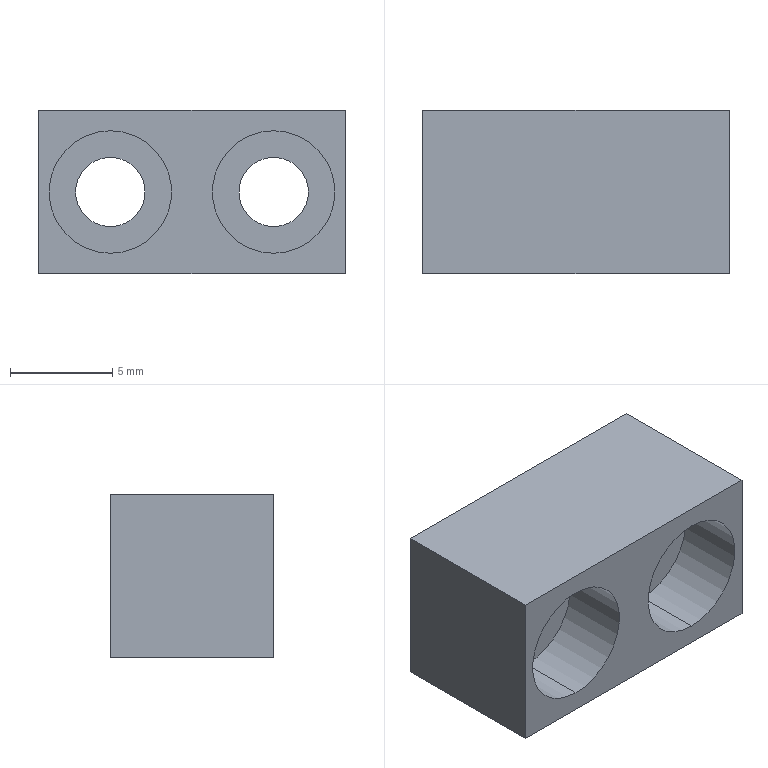Part | NX | features BREP 1 | 1 solid | 19 faces | box 15 x 8 x 8 mm | volume 660.349 mm3 | cylinder 10 | plane 9 | commonest cylinder face diameters 3.4 x4 6 x4 4.5 x2
STEP:
#1=CARTESIAN_POINT('',(4.,-0.6,3.));
#2=VERTEX_POINT('',#1);
#3=CARTESIAN_POINT('',(4.,-0.6,-3.));
#4=VERTEX_POINT('',#3);
#5=CARTESIAN_POINT('',(4.,-0.6,0.));
#6=DIRECTION('',(0.,-1.,0.));
#7=DIRECTION('',(0.,0.,-1.));
#8=AXIS2_PLACEMENT_3D('',#5,#6,#7);
#9=CIRCLE('',#8,3.);
#10=EDGE_CURVE('',#2,#4,#9,.T.);
#11=ORIENTED_EDGE('',*,*,#10,.F.);
#12=CARTESIAN_POINT('',(4.,-4.,3.));
#13=VERTEX_POINT('',#12);
#14=CARTESIAN_POINT('',(4.,-4.,3.));
#15=DIRECTION('',(0.,-1.,0.));
#16=VECTOR('',#15,1000.);
#17=LINE('',#14,#16);
#18=EDGE_CURVE('',#13,#2,#17,.F.);
#19=ORIENTED_EDGE('',*,*,#18,.F.);
#20=CARTESIAN_POINT('',(4.,-4.,-3.));
#21=VERTEX_POINT('',#20);
#22=CARTESIAN_POINT('',(4.,-4.,0.));
#23=DIRECTION('',(0.,-1.,0.));
#24=DIRECTION('',(0.,0.,-1.));
#25=AXIS2_PLACEMENT_3D('',#22,#23,#24);
#26=CIRCLE('',#25,3.);
#27=EDGE_CURVE('',#13,#21,#26,.T.);
#28=ORIENTED_EDGE('',*,*,#27,.T.);
#29=CARTESIAN_POINT('',(4.,-4.,-3.));
#30=DIRECTION('',(0.,-1.,0.));
#31=VECTOR('',#30,1000.);
#32=LINE('',#29,#31);
#33=EDGE_CURVE('',#21,#4,#32,.F.);
#34=ORIENTED_EDGE('',*,*,#33,.T.);
#35=EDGE_LOOP('',(#11,#19,#28,#34));
#36=FACE_BOUND('',#35,.T.);
#37=CARTESIAN_POINT('',(4.,-4.,0.));
#38=DIRECTION('',(0.,-1.,0.));
#39=DIRECTION('',(0.,0.,1.));
#40=AXIS2_PLACEMENT_3D('',#37,#38,#39);
#41=CYLINDRICAL_SURFACE('',#40,3.);
#42=ADVANCED_FACE('',(#36),#41,.F.);
#43=CARTESIAN_POINT('',(4.,4.,1.7));
#44=VERTEX_POINT('',#43);
#45=CARTESIAN_POINT('',(4.,4.,-1.7));
#46=VERTEX_POINT('',#45);
#47=CARTESIAN_POINT('',(4.,4.,0.));
#48=DIRECTION('',(0.,-1.,0.));
#49=DIRECTION('',(0.,0.,-1.));
#50=AXIS2_PLACEMENT_3D('',#47,#48,#49);
#51=CIRCLE('',#50,1.7);
#52=EDGE_CURVE('',#44,#46,#51,.T.);
#53=ORIENTED_EDGE('',*,*,#52,.F.);
#54=CARTESIAN_POINT('',(4.,-0.6,1.7));
#55=VERTEX_POINT('',#54);
#56=CARTESIAN_POINT('',(4.,-4.,1.7));
#57=DIRECTION('',(0.,-1.,0.));
#58=VECTOR('',#57,1000.);
#59=LINE('',#56,#58);
#60=EDGE_CURVE('',#55,#44,#59,.F.);
#61=ORIENTED_EDGE('',*,*,#60,.F.);
#62=CARTESIAN_POINT('',(4.,-0.6,-1.7));
#63=VERTEX_POINT('',#62);
#64=CARTESIAN_POINT('',(4.,-0.6,0.));
#65=DIRECTION('',(0.,-1.,0.));
#66=DIRECTION('',(0.,0.,-1.));
#67=AXIS2_PLACEMENT_3D('',#64,#65,#66);
#68=CIRCLE('',#67,1.7);
#69=EDGE_CURVE('',#55,#63,#68,.T.);
#70=ORIENTED_EDGE('',*,*,#69,.T.);
#71=CARTESIAN_POINT('',(4.,-4.,-1.7));
#72=DIRECTION('',(0.,-1.,0.));
#73=VECTOR('',#72,1000.);
#74=LINE('',#71,#73);
#75=EDGE_CURVE('',#63,#46,#74,.F.);
#76=ORIENTED_EDGE('',*,*,#75,.T.);
#77=EDGE_LOOP('',(#53,#61,#70,#76));
#78=FACE_BOUND('',#77,.T.);
#79=CARTESIAN_POINT('',(4.,-4.,0.));
#80=DIRECTION('',(0.,-1.,0.));
#81=DIRECTION('',(0.,0.,1.));
#82=AXIS2_PLACEMENT_3D('',#79,#80,#81);
#83=CYLINDRICAL_SURFACE('',#82,1.7);
#84=ADVANCED_FACE('',(#78),#83,.F.);
#85=CARTESIAN_POINT('',(-4.,-0.6,3.));
#86=VERTEX_POINT('',#85);
#87=CARTESIAN_POINT('',(-4.,-0.6,-3.));
#88=VERTEX_POINT('',#87);
#89=CARTESIAN_POINT('',(-4.,-0.6,0.));
#90=DIRECTION('',(0.,-1.,0.));
#91=DIRECTION('',(0.,0.,-1.));
#92=AXIS2_PLACEMENT_3D('',#89,#90,#91);
#93=CIRCLE('',#92,3.);
#94=EDGE_CURVE('',#86,#88,#93,.T.);
#95=ORIENTED_EDGE('',*,*,#94,.F.);
#96=CARTESIAN_POINT('',(-4.,-4.,3.));
#97=VERTEX_POINT('',#96);
#98=CARTESIAN_POINT('',(-4.,-4.,3.));
#99=DIRECTION('',(0.,-1.,0.));
#100=VECTOR('',#99,1000.);
#101=LINE('',#98,#100);
#102=EDGE_CURVE('',#97,#86,#101,.F.);
#103=ORIENTED_EDGE('',*,*,#102,.F.);
#104=CARTESIAN_POINT('',(-4.,-4.,-3.));
#105=VERTEX_POINT('',#104);
#106=CARTESIAN_POINT('',(-4.,-4.,0.));
#107=DIRECTION('',(0.,-1.,0.));
#108=DIRECTION('',(0.,0.,-1.));
#109=AXIS2_PLACEMENT_3D('',#106,#107,#108);
#110=CIRCLE('',#109,3.);
#111=EDGE_CURVE('',#97,#105,#110,.T.);
#112=ORIENTED_EDGE('',*,*,#111,.T.);
#113=CARTESIAN_POINT('',(-4.,-4.,-3.));
#114=DIRECTION('',(0.,-1.,0.));
#115=VECTOR('',#114,1000.);
#116=LINE('',#113,#115);
#117=EDGE_CURVE('',#105,#88,#116,.F.);
#118=ORIENTED_EDGE('',*,*,#117,.T.);
#119=EDGE_LOOP('',(#95,#103,#112,#118));
#120=FACE_BOUND('',#119,.T.);
#121=CARTESIAN_POINT('',(-4.,-4.,0.));
#122=DIRECTION('',(0.,-1.,0.));
#123=DIRECTION('',(0.,0.,1.));
#124=AXIS2_PLACEMENT_3D('',#121,#122,#123);
#125=CYLINDRICAL_SURFACE('',#124,3.);
#126=ADVANCED_FACE('',(#120),#125,.F.);
#127=CARTESIAN_POINT('',(-4.,4.,1.7));
#128=VERTEX_POINT('',#127);
#129=CARTESIAN_POINT('',(-4.,4.,-1.7));
#130=VERTEX_POINT('',#129);
#131=CARTESIAN_POINT('',(-4.,4.,0.));
#132=DIRECTION('',(0.,-1.,0.));
#133=DIRECTION('',(0.,0.,-1.));
#134=AXIS2_PLACEMENT_3D('',#131,#132,#133);
#135=CIRCLE('',#134,1.7);
#136=EDGE_CURVE('',#128,#130,#135,.T.);
#137=ORIENTED_EDGE('',*,*,#136,.F.);
#138=CARTESIAN_POINT('',(-4.,-0.6,1.7));
#139=VERTEX_POINT('',#138);
#140=CARTESIAN_POINT('',(-4.,-4.,1.7));
#141=DIRECTION('',(0.,-1.,0.));
#142=VECTOR('',#141,1000.);
#143=LINE('',#140,#142);
#144=EDGE_CURVE('',#139,#128,#143,.F.);
#145=ORIENTED_EDGE('',*,*,#144,.F.);
#146=CARTESIAN_POINT('',(-4.,-0.6,-1.7));
#147=VERTEX_POINT('',#146);
#148=CARTESIAN_POINT('',(-4.,-0.6,0.));
#149=DIRECTION('',(0.,-1.,0.));
#150=DIRECTION('',(0.,0.,-1.));
#151=AXIS2_PLACEMENT_3D('',#148,#149,#150);
#152=CIRCLE('',#151,1.7);
#153=EDGE_CURVE('',#139,#147,#152,.T.);
#154=ORIENTED_EDGE('',*,*,#153,.T.);
#155=CARTESIAN_POINT('',(-4.,-4.,-1.7));
#156=DIRECTION('',(0.,-1.,0.));
#157=VECTOR('',#156,1000.);
#158=LINE('',#155,#157);
#159=EDGE_CURVE('',#147,#130,#158,.F.);
#160=ORIENTED_EDGE('',*,*,#159,.T.);
#161=EDGE_LOOP('',(#137,#145,#154,#160));
#162=FACE_BOUND('',#161,.T.);
#163=CARTESIAN_POINT('',(-4.,-4.,0.));
#164=DIRECTION('',(0.,-1.,0.));
#165=DIRECTION('',(0.,0.,1.));
#166=AXIS2_PLACEMENT_3D('',#163,#164,#165);
#167=CYLINDRICAL_SURFACE('',#166,1.7);
#168=ADVANCED_FACE('',(#162),#167,.F.);
#169=CARTESIAN_POINT('',(2.25,1.,-2.5));
#170=VERTEX_POINT('',#169);
#171=CARTESIAN_POINT('',(-2.25,1.,-2.5));
#172=VERTEX_POINT('',#171);
#173=CARTESIAN_POINT('',(0.,1.,-2.5));
#174=DIRECTION('',(0.,0.,-1.));
#175=DIRECTION('',(-1.,0.,0.));
#176=AXIS2_PLACEMENT_3D('',#173,#174,#175);
#177=CIRCLE('',#176,2.25);
#178=EDGE_CURVE('',#170,#172,#177,.T.);
#179=ORIENTED_EDGE('',*,*,#178,.F.);
#180=CARTESIAN_POINT('',(2.25,1.,-4.));
#181=VERTEX_POINT('',#180);
#182=CARTESIAN_POINT('',(2.25,1.,-2.5));
#183=DIRECTION('',(0.,0.,-1.));
#184=VECTOR('',#183,1000.);
#185=LINE('',#182,#184);
#186=EDGE_CURVE('',#181,#170,#185,.F.);
#187=ORIENTED_EDGE('',*,*,#186,.F.);
#188=CARTESIAN_POINT('',(-2.25,1.,-4.));
#189=VERTEX_POINT('',#188);
#190=CARTESIAN_POINT('',(0.,1.,-4.));
#191=DIRECTION('',(0.,0.,-1.));
#192=DIRECTION('',(-1.,0.,0.));
#193=AXIS2_PLACEMENT_3D('',#190,#191,#192);
#194=CIRCLE('',#193,2.25);
#195=EDGE_CURVE('',#181,#189,#194,.T.);
#196=ORIENTED_EDGE('',*,*,#195,.T.);
#197=CARTESIAN_POINT('',(-2.25,1.,-2.5));
#198=DIRECTION('',(0.,0.,-1.));
#199=VECTOR('',#198,1000.);
#200=LINE('',#197,#199);
#201=EDGE_CURVE('',#189,#172,#200,.F.);
#202=ORIENTED_EDGE('',*,*,#201,.T.);
#203=EDGE_LOOP('',(#179,#187,#196,#202));
#204=FACE_BOUND('',#203,.T.);
#205=CARTESIAN_POINT('',(0.,1.,-2.5));
#206=DIRECTION('',(0.,0.,-1.));
#207=DIRECTION('',(1.,0.,0.));
#208=AXIS2_PLACEMENT_3D('',#205,#206,#207);
#209=CYLINDRICAL_SURFACE('',#208,2.25);
#210=ADVANCED_FACE('',(#204),#209,.F.);
#211=CARTESIAN_POINT('',(7.5,-4.,-4.));
#212=VERTEX_POINT('',#211);
#213=CARTESIAN_POINT('',(7.5,4.,-4.));
#214=VERTEX_POINT('',#213);
#215=CARTESIAN_POINT('',(7.5,4.,-4.));
#216=DIRECTION('',(0.,1.,0.));
#217=VECTOR('',#216,1000.);
#218=LINE('',#215,#217);
#219=EDGE_CURVE('',#212,#214,#218,.T.);
#220=ORIENTED_EDGE('',*,*,#219,.T.);
#221=CARTESIAN_POINT('',(7.5,4.,4.));
#222=VERTEX_POINT('',#221);
#223=CARTESIAN_POINT('',(7.5,4.,4.));
#224=DIRECTION('',(0.,0.,-1.));
#225=VECTOR('',#224,1000.);
#226=LINE('',#223,#225);
#227=EDGE_CURVE('',#222,#214,#226,.T.);
#228=ORIENTED_EDGE('',*,*,#227,.F.);
#229=CARTESIAN_POINT('',(7.5,-4.,4.));
#230=VERTEX_POINT('',#229);
#231=CARTESIAN_POINT('',(7.5,4.,4.));
#232=DIRECTION('',(0.,1.,0.));
#233=VECTOR('',#232,1000.);
#234=LINE('',#231,#233);
#235=EDGE_CURVE('',#230,#222,#234,.T.);
#236=ORIENTED_EDGE('',*,*,#235,.F.);
#237=CARTESIAN_POINT('',(7.5,-4.,4.));
#238=DIRECTION('',(0.,0.,-1.));
#239=VECTOR('',#238,1000.);
#240=LINE('',#237,#239);
#241=EDGE_CURVE('',#230,#212,#240,.T.);
#242=ORIENTED_EDGE('',*,*,#241,.T.);
#243=EDGE_LOOP('',(#220,#228,#236,#242));
#244=FACE_BOUND('',#243,.T.);
#245=CARTESIAN_POINT('',(7.5,4.,4.));
#246=DIRECTION('',(-1.,0.,0.));
#247=DIRECTION('',(0.,0.,-1.));
#248=AXIS2_PLACEMENT_3D('',#245,#246,#247);
#249=PLANE('',#248);
#250=ADVANCED_FACE('',(#244),#249,.F.);
#251=CARTESIAN_POINT('',(4.,4.,0.));
#252=DIRECTION('',(0.,-1.,0.));
#253=DIRECTION('',(0.,0.,-1.));
#254=AXIS2_PLACEMENT_3D('',#251,#252,#253);
#255=CIRCLE('',#254,1.7);
#256=EDGE_CURVE('',#46,#44,#255,.T.);
#257=ORIENTED_EDGE('',*,*,#256,.T.);
#258=ORIENTED_EDGE('',*,*,#52,.T.);
#259=EDGE_LOOP('',(#257,#258));
#260=FACE_BOUND('',#259,.T.);
#261=CARTESIAN_POINT('',(-4.,4.,0.));
#262=DIRECTION('',(0.,-1.,0.));
#263=DIRECTION('',(0.,0.,-1.));
#264=AXIS2_PLACEMENT_3D('',#261,#262,#263);
#265=CIRCLE('',#264,1.7);
#266=EDGE_CURVE('',#130,#128,#265,.T.);
#267=ORIENTED_EDGE('',*,*,#266,.T.);
#268=ORIENTED_EDGE('',*,*,#136,.T.);
#269=EDGE_LOOP('',(#267,#268));
#270=FACE_BOUND('',#269,.T.);
#271=CARTESIAN_POINT('',(-7.5,4.,-4.));
#272=VERTEX_POINT('',#271);
#273=CARTESIAN_POINT('',(-7.5,4.,-4.));
#274=DIRECTION('',(-1.,0.,0.));
#275=VECTOR('',#274,1000.);
#276=LINE('',#273,#275);
#277=EDGE_CURVE('',#214,#272,#276,.T.);
#278=ORIENTED_EDGE('',*,*,#277,.T.);
#279=CARTESIAN_POINT('',(-7.5,4.,4.));
#280=VERTEX_POINT('',#279);
#281=CARTESIAN_POINT('',(-7.5,4.,4.));
#282=DIRECTION('',(0.,0.,-1.));
#283=VECTOR('',#282,1000.);
#284=LINE('',#281,#283);
#285=EDGE_CURVE('',#280,#272,#284,.T.);
#286=ORIENTED_EDGE('',*,*,#285,.F.);
#287=CARTESIAN_POINT('',(-7.5,4.,4.));
#288=DIRECTION('',(-1.,0.,0.));
#289=VECTOR('',#288,1000.);
#290=LINE('',#287,#289);
#291=EDGE_CURVE('',#222,#280,#290,.T.);
#292=ORIENTED_EDGE('',*,*,#291,.F.);
#293=ORIENTED_EDGE('',*,*,#227,.T.);
#294=EDGE_LOOP('',(#278,#286,#292,#293));
#295=FACE_BOUND('',#294,.T.);
#296=CARTESIAN_POINT('',(-7.5,4.,4.));
#297=DIRECTION('',(0.,-1.,0.));
#298=DIRECTION('',(0.,0.,1.));
#299=AXIS2_PLACEMENT_3D('',#296,#297,#298);
#300=PLANE('',#299);
#301=ADVANCED_FACE('',(#260,#270,#295),#300,.F.);
#302=CARTESIAN_POINT('',(-7.5,-4.,-4.));
#303=VERTEX_POINT('',#302);
#304=CARTESIAN_POINT('',(-7.5,4.,-4.));
#305=DIRECTION('',(0.,-1.,0.));
#306=VECTOR('',#305,1000.);
#307=LINE('',#304,#306);
#308=EDGE_CURVE('',#272,#303,#307,.T.);
#309=ORIENTED_EDGE('',*,*,#308,.T.);
#310=CARTESIAN_POINT('',(-7.5,-4.,4.));
#311=VERTEX_POINT('',#310);
#312=CARTESIAN_POINT('',(-7.5,-4.,4.));
#313=DIRECTION('',(0.,0.,-1.));
#314=VECTOR('',#313,1000.);
#315=LINE('',#312,#314);
#316=EDGE_CURVE('',#311,#303,#315,.T.);
#317=ORIENTED_EDGE('',*,*,#316,.F.);
#318=CARTESIAN_POINT('',(-7.5,4.,4.));
#319=DIRECTION('',(0.,-1.,0.));
#320=VECTOR('',#319,1000.);
#321=LINE('',#318,#320);
#322=EDGE_CURVE('',#280,#311,#321,.T.);
#323=ORIENTED_EDGE('',*,*,#322,.F.);
#324=ORIENTED_EDGE('',*,*,#285,.T.);
#325=EDGE_LOOP('',(#309,#317,#323,#324));
#326=FACE_BOUND('',#325,.T.);
#327=CARTESIAN_POINT('',(-7.5,4.,4.));
#328=DIRECTION('',(1.,0.,0.));
#329=DIRECTION('',(0.,-1.,0.));
#330=AXIS2_PLACEMENT_3D('',#327,#328,#329);
#331=PLANE('',#330);
#332=ADVANCED_FACE('',(#326),#331,.F.);
#333=CARTESIAN_POINT('',(4.,-4.,0.));
#334=DIRECTION('',(0.,-1.,0.));
#335=DIRECTION('',(0.,0.,-1.));
#336=AXIS2_PLACEMENT_3D('',#333,#334,#335);
#337=CIRCLE('',#336,3.);
#338=EDGE_CURVE('',#21,#13,#337,.T.);
#339=ORIENTED_EDGE('',*,*,#338,.F.);
#340=ORIENTED_EDGE('',*,*,#27,.F.);
#341=EDGE_LOOP('',(#339,#340));
#342=FACE_BOUND('',#341,.T.);
#343=CARTESIAN_POINT('',(-4.,-4.,0.));
#344=DIRECTION('',(0.,-1.,0.));
#345=DIRECTION('',(0.,0.,-1.));
#346=AXIS2_PLACEMENT_3D('',#343,#344,#345);
#347=CIRCLE('',#346,3.);
#348=EDGE_CURVE('',#105,#97,#347,.T.);
#349=ORIENTED_EDGE('',*,*,#348,.F.);
#350=ORIENTED_EDGE('',*,*,#111,.F.);
#351=EDGE_LOOP('',(#349,#350));
#352=FACE_BOUND('',#351,.T.);
#353=CARTESIAN_POINT('',(-7.5,-4.,-4.));
#354=DIRECTION('',(1.,0.,0.));
#355=VECTOR('',#354,1000.);
#356=LINE('',#353,#355);
#357=EDGE_CURVE('',#303,#212,#356,.T.);
#358=ORIENTED_EDGE('',*,*,#357,.T.);
#359=ORIENTED_EDGE('',*,*,#241,.F.);
#360=CARTESIAN_POINT('',(-7.5,-4.,4.));
#361=DIRECTION('',(1.,0.,0.));
#362=VECTOR('',#361,1000.);
#363=LINE('',#360,#362);
#364=EDGE_CURVE('',#311,#230,#363,.T.);
#365=ORIENTED_EDGE('',*,*,#364,.F.);
#366=ORIENTED_EDGE('',*,*,#316,.T.);
#367=EDGE_LOOP('',(#358,#359,#365,#366));
#368=FACE_BOUND('',#367,.T.);
#369=CARTESIAN_POINT('',(-7.5,-4.,4.));
#370=DIRECTION('',(0.,1.,0.));
#371=DIRECTION('',(0.,0.,-1.));
#372=AXIS2_PLACEMENT_3D('',#369,#370,#371);
#373=PLANE('',#372);
#374=ADVANCED_FACE('',(#342,#352,#368),#373,.F.);
#375=ORIENTED_EDGE('',*,*,#235,.T.);
#376=ORIENTED_EDGE('',*,*,#291,.T.);
#377=ORIENTED_EDGE('',*,*,#322,.T.);
#378=ORIENTED_EDGE('',*,*,#364,.T.);
#379=EDGE_LOOP('',(#375,#376,#377,#378));
#380=FACE_BOUND('',#379,.T.);
#381=CARTESIAN_POINT('',(0.,0.,4.));
#382=DIRECTION('',(0.,0.,1.));
#383=DIRECTION('',(-1.,0.,0.));
#384=AXIS2_PLACEMENT_3D('',#381,#382,#383);
#385=PLANE('',#384);
#386=ADVANCED_FACE('',(#380),#385,.T.);
#387=CARTESIAN_POINT('',(0.,1.,-4.));
#388=DIRECTION('',(0.,0.,-1.));
#389=DIRECTION('',(-1.,0.,0.));
#390=AXIS2_PLACEMENT_3D('',#387,#388,#389);
#391=CIRCLE('',#390,2.25);
#392=EDGE_CURVE('',#189,#181,#391,.T.);
#393=ORIENTED_EDGE('',*,*,#392,.F.);
#394=ORIENTED_EDGE('',*,*,#195,.F.);
#395=EDGE_LOOP('',(#393,#394));
#396=FACE_BOUND('',#395,.T.);
#397=ORIENTED_EDGE('',*,*,#219,.F.);
#398=ORIENTED_EDGE('',*,*,#357,.F.);
#399=ORIENTED_EDGE('',*,*,#308,.F.);
#400=ORIENTED_EDGE('',*,*,#277,.F.);
#401=EDGE_LOOP('',(#397,#398,#399,#400));
#402=FACE_BOUND('',#401,.T.);
#403=CARTESIAN_POINT('',(0.,0.,-4.));
#404=DIRECTION('',(0.,0.,1.));
#405=DIRECTION('',(-1.,0.,0.));
#406=AXIS2_PLACEMENT_3D('',#403,#404,#405);
#407=PLANE('',#406);
#408=ADVANCED_FACE('',(#396,#402),#407,.F.);
#409=ORIENTED_EDGE('',*,*,#186,.T.);
#410=CARTESIAN_POINT('',(0.,1.,-2.5));
#411=DIRECTION('',(0.,0.,-1.));
#412=DIRECTION('',(-1.,0.,0.));
#413=AXIS2_PLACEMENT_3D('',#410,#411,#412);
#414=CIRCLE('',#413,2.25);
#415=EDGE_CURVE('',#172,#170,#414,.T.);
#416=ORIENTED_EDGE('',*,*,#415,.F.);
#417=ORIENTED_EDGE('',*,*,#201,.F.);
#418=ORIENTED_EDGE('',*,*,#392,.T.);
#419=EDGE_LOOP('',(#409,#416,#417,#418));
#420=FACE_BOUND('',#419,.T.);
#421=CARTESIAN_POINT('',(0.,1.,-2.5));
#422=DIRECTION('',(0.,0.,-1.));
#423=DIRECTION('',(1.,0.,0.));
#424=AXIS2_PLACEMENT_3D('',#421,#422,#423);
#425=CYLINDRICAL_SURFACE('',#424,2.25);
#426=ADVANCED_FACE('',(#420),#425,.F.);
#427=ORIENTED_EDGE('',*,*,#415,.T.);
#428=ORIENTED_EDGE('',*,*,#178,.T.);
#429=EDGE_LOOP('',(#427,#428));
#430=FACE_BOUND('',#429,.T.);
#431=CARTESIAN_POINT('',(0.,1.,-2.5));
#432=DIRECTION('',(0.,0.,-1.));
#433=DIRECTION('',(1.,0.,0.));
#434=AXIS2_PLACEMENT_3D('',#431,#432,#433);
#435=PLANE('',#434);
#436=ADVANCED_FACE('',(#430),#435,.T.);
#437=ORIENTED_EDGE('',*,*,#144,.T.);
#438=ORIENTED_EDGE('',*,*,#266,.F.);
#439=ORIENTED_EDGE('',*,*,#159,.F.);
#440=CARTESIAN_POINT('',(-4.,-0.6,0.));
#441=DIRECTION('',(0.,-1.,0.));
#442=DIRECTION('',(0.,0.,-1.));
#443=AXIS2_PLACEMENT_3D('',#440,#441,#442);
#444=CIRCLE('',#443,1.7);
#445=EDGE_CURVE('',#147,#139,#444,.T.);
#446=ORIENTED_EDGE('',*,*,#445,.T.);
#447=EDGE_LOOP('',(#437,#438,#439,#446));
#448=FACE_BOUND('',#447,.T.);
#449=CARTESIAN_POINT('',(-4.,-4.,0.));
#450=DIRECTION('',(0.,-1.,0.));
#451=DIRECTION('',(0.,0.,1.));
#452=AXIS2_PLACEMENT_3D('',#449,#450,#451);
#453=CYLINDRICAL_SURFACE('',#452,1.7);
#454=ADVANCED_FACE('',(#448),#453,.F.);
#455=ORIENTED_EDGE('',*,*,#445,.F.);
#456=ORIENTED_EDGE('',*,*,#153,.F.);
#457=EDGE_LOOP('',(#455,#456));
#458=FACE_BOUND('',#457,.T.);
#459=CARTESIAN_POINT('',(-4.,-0.6,0.));
#460=DIRECTION('',(0.,-1.,0.));
#461=DIRECTION('',(0.,0.,-1.));
#462=AXIS2_PLACEMENT_3D('',#459,#460,#461);
#463=CIRCLE('',#462,3.);
#464=EDGE_CURVE('',#88,#86,#463,.T.);
#465=ORIENTED_EDGE('',*,*,#464,.T.);
#466=ORIENTED_EDGE('',*,*,#94,.T.);
#467=EDGE_LOOP('',(#465,#466));
#468=FACE_BOUND('',#467,.T.);
#469=CARTESIAN_POINT('',(-2.3,-0.6,0.));
#470=DIRECTION('',(0.,1.,0.));
#471=DIRECTION('',(0.,0.,-1.));
#472=AXIS2_PLACEMENT_3D('',#469,#470,#471);
#473=PLANE('',#472);
#474=ADVANCED_FACE('',(#458,#468),#473,.F.);
#475=ORIENTED_EDGE('',*,*,#102,.T.);
#476=ORIENTED_EDGE('',*,*,#464,.F.);
#477=ORIENTED_EDGE('',*,*,#117,.F.);
#478=ORIENTED_EDGE('',*,*,#348,.T.);
#479=EDGE_LOOP('',(#475,#476,#477,#478));
#480=FACE_BOUND('',#479,.T.);
#481=CARTESIAN_POINT('',(-4.,-4.,0.));
#482=DIRECTION('',(0.,-1.,0.));
#483=DIRECTION('',(0.,0.,1.));
#484=AXIS2_PLACEMENT_3D('',#481,#482,#483);
#485=CYLINDRICAL_SURFACE('',#484,3.);
#486=ADVANCED_FACE('',(#480),#485,.F.);
#487=ORIENTED_EDGE('',*,*,#60,.T.);
#488=ORIENTED_EDGE('',*,*,#256,.F.);
#489=ORIENTED_EDGE('',*,*,#75,.F.);
#490=CARTESIAN_POINT('',(4.,-0.6,0.));
#491=DIRECTION('',(0.,-1.,0.));
#492=DIRECTION('',(0.,0.,-1.));
#493=AXIS2_PLACEMENT_3D('',#490,#491,#492);
#494=CIRCLE('',#493,1.7);
#495=EDGE_CURVE('',#63,#55,#494,.T.);
#496=ORIENTED_EDGE('',*,*,#495,.T.);
#497=EDGE_LOOP('',(#487,#488,#489,#496));
#498=FACE_BOUND('',#497,.T.);
#499=CARTESIAN_POINT('',(4.,-4.,0.));
#500=DIRECTION('',(0.,-1.,0.));
#501=DIRECTION('',(0.,0.,1.));
#502=AXIS2_PLACEMENT_3D('',#499,#500,#501);
#503=CYLINDRICAL_SURFACE('',#502,1.7);
#504=ADVANCED_FACE('',(#498),#503,.F.);
#505=ORIENTED_EDGE('',*,*,#495,.F.);
#506=ORIENTED_EDGE('',*,*,#69,.F.);
#507=EDGE_LOOP('',(#505,#506));
#508=FACE_BOUND('',#507,.T.);
#509=CARTESIAN_POINT('',(4.,-0.6,0.));
#510=DIRECTION('',(0.,-1.,0.));
#511=DIRECTION('',(0.,0.,-1.));
#512=AXIS2_PLACEMENT_3D('',#509,#510,#511);
#513=CIRCLE('',#512,3.);
#514=EDGE_CURVE('',#4,#2,#513,.T.);
#515=ORIENTED_EDGE('',*,*,#514,.T.);
#516=ORIENTED_EDGE('',*,*,#10,.T.);
#517=EDGE_LOOP('',(#515,#516));
#518=FACE_BOUND('',#517,.T.);
#519=CARTESIAN_POINT('',(5.7,-0.6,0.));
#520=DIRECTION('',(0.,1.,0.));
#521=DIRECTION('',(0.,0.,-1.));
#522=AXIS2_PLACEMENT_3D('',#519,#520,#521);
#523=PLANE('',#522);
#524=ADVANCED_FACE('',(#508,#518),#523,.F.);
#525=ORIENTED_EDGE('',*,*,#18,.T.);
#526=ORIENTED_EDGE('',*,*,#514,.F.);
#527=ORIENTED_EDGE('',*,*,#33,.F.);
#528=ORIENTED_EDGE('',*,*,#338,.T.);
#529=EDGE_LOOP('',(#525,#526,#527,#528));
#530=FACE_BOUND('',#529,.T.);
#531=CARTESIAN_POINT('',(4.,-4.,0.));
#532=DIRECTION('',(0.,-1.,0.));
#533=DIRECTION('',(0.,0.,1.));
#534=AXIS2_PLACEMENT_3D('',#531,#532,#533);
#535=CYLINDRICAL_SURFACE('',#534,3.);
#536=ADVANCED_FACE('',(#530),#535,.F.);
#537=CLOSED_SHELL('',(#42,#84,#126,#168,#210,#250,#301,#332,#374,#386,#408,#426,#436,#454,#474,#486,#504,#524,#536));
#538=MANIFOLD_SOLID_BREP('',#537);
#539=(LENGTH_UNIT()NAMED_UNIT(*)SI_UNIT(.MILLI.,.METRE.));
#540=UNCERTAINTY_MEASURE_WITH_UNIT(LENGTH_MEASURE(0.00001),#539,'','');
#541=(NAMED_UNIT(*)PLANE_ANGLE_UNIT()SI_UNIT($,.RADIAN.));
#542=(NAMED_UNIT(*)SI_UNIT($,.STERADIAN.)SOLID_ANGLE_UNIT());
#543=(GEOMETRIC_REPRESENTATION_CONTEXT(3)GLOBAL_UNCERTAINTY_ASSIGNED_CONTEXT((#540))GLOBAL_UNIT_ASSIGNED_CONTEXT((#539,#541,#542))REPRESENTATION_CONTEXT('',''));
#544=ADVANCED_BREP_SHAPE_REPRESENTATION('',(#538),#543);